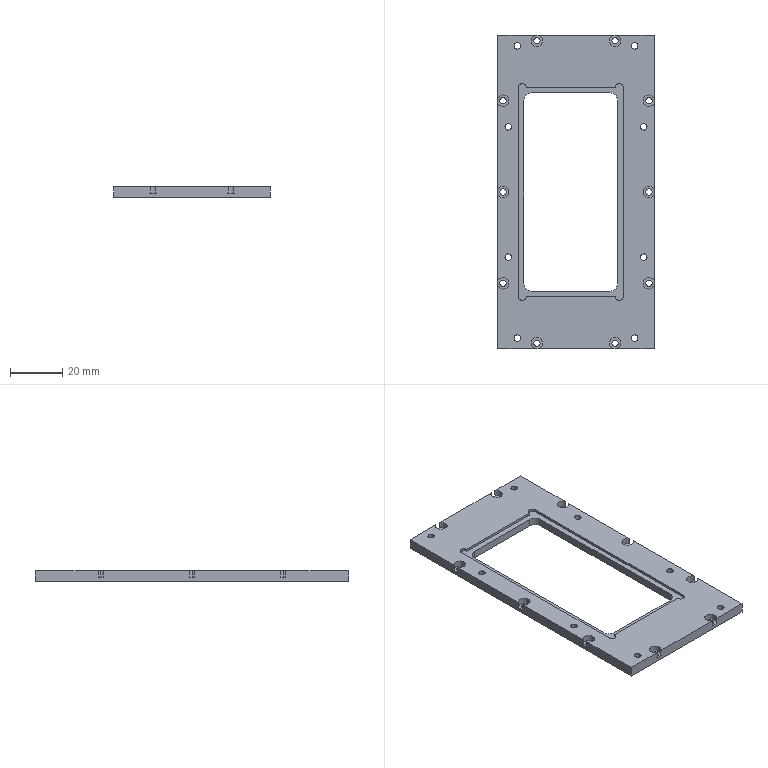Part | 1 solid | 90 faces | box 60 x 120 x 4 mm | volume 16789 mm3 | cylinder 65 | plane 25 | commonest cylinder face diameters 4.4 x21 2.4 x20 2.5 x16 3 x4 6 x4